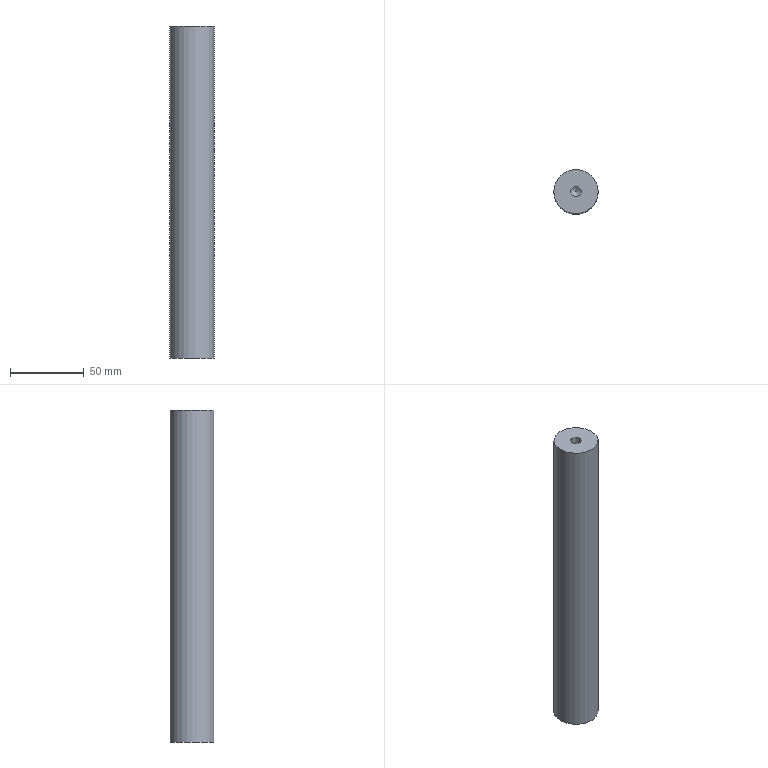Part | NX | features solid 2 | 1 solid | 7 faces | box 30 x 30 x 225 mm | volume 156299 mm3 | cylinder 3 | plane 2 | cone 2 | commonest cylinder face diameters 6.985 x1 8.782 x1 30 x1
STEP:
#1=CARTESIAN_POINT('',(243.507,265.,-170.));
#2=VERTEX_POINT('',#1);
#3=CARTESIAN_POINT('',(247.,265.,-170.));
#4=DIRECTION('',(0.,0.,-1.));
#5=DIRECTION('',(-1.,0.,0.));
#6=AXIS2_PLACEMENT_3D('',#3,#4,#5);
#7=CIRCLE('',#6,3.493);
#8=EDGE_CURVE('',#2,#2,#7,.T.);
#9=ORIENTED_EDGE('',*,*,#8,.T.);
#10=EDGE_LOOP('',(#9));
#11=FACE_BOUND('',#10,.T.);
#12=CARTESIAN_POINT('',(232.,265.,-170.));
#13=VERTEX_POINT('',#12);
#14=CARTESIAN_POINT('',(247.,265.,-170.));
#15=DIRECTION('',(0.,0.,-1.));
#16=DIRECTION('',(-1.,0.,0.));
#17=AXIS2_PLACEMENT_3D('',#14,#15,#16);
#18=CIRCLE('',#17,15.);
#19=EDGE_CURVE('',#13,#13,#18,.T.);
#20=ORIENTED_EDGE('',*,*,#19,.F.);
#21=EDGE_LOOP('',(#20));
#22=FACE_BOUND('',#21,.T.);
#23=CARTESIAN_POINT('',(247.,285.,-170.));
#24=DIRECTION('',(0.,0.,-1.));
#25=DIRECTION('',(-1.,0.,0.));
#26=AXIS2_PLACEMENT_3D('',#23,#24,#25);
#27=PLANE('',#26);
#28=ADVANCED_FACE('',(#11,#22),#27,.F.);
#29=CARTESIAN_POINT('',(232.,265.,-395.));
#30=VERTEX_POINT('',#29);
#31=CARTESIAN_POINT('',(247.,265.,-395.));
#32=DIRECTION('',(0.,0.,-1.));
#33=DIRECTION('',(-1.,0.,0.));
#34=AXIS2_PLACEMENT_3D('',#31,#32,#33);
#35=CIRCLE('',#34,15.);
#36=EDGE_CURVE('',#30,#30,#35,.T.);
#37=ORIENTED_EDGE('',*,*,#36,.F.);
#38=EDGE_LOOP('',(#37));
#39=FACE_BOUND('',#38,.T.);
#40=ORIENTED_EDGE('',*,*,#19,.T.);
#41=EDGE_LOOP('',(#40));
#42=FACE_BOUND('',#41,.T.);
#43=CARTESIAN_POINT('',(247.,265.,-250.));
#44=DIRECTION('',(0.,0.,-1.));
#45=DIRECTION('',(-1.,0.,0.));
#46=AXIS2_PLACEMENT_3D('',#43,#44,#45);
#47=CYLINDRICAL_SURFACE('',#46,15.);
#48=ADVANCED_FACE('',(#39,#42),#47,.T.);
#49=CARTESIAN_POINT('',(251.391,265.,-395.));
#50=VERTEX_POINT('',#49);
#51=CARTESIAN_POINT('',(247.,265.,-395.));
#52=DIRECTION('',(0.,0.,1.));
#53=DIRECTION('',(1.,0.,0.));
#54=AXIS2_PLACEMENT_3D('',#51,#52,#53);
#55=CIRCLE('',#54,4.391);
#56=EDGE_CURVE('',#50,#50,#55,.T.);
#57=ORIENTED_EDGE('',*,*,#56,.T.);
#58=EDGE_LOOP('',(#57));
#59=FACE_BOUND('',#58,.T.);
#60=ORIENTED_EDGE('',*,*,#36,.T.);
#61=EDGE_LOOP('',(#60));
#62=FACE_BOUND('',#61,.T.);
#63=CARTESIAN_POINT('',(247.,265.,-395.));
#64=DIRECTION('',(0.,0.,-1.));
#65=DIRECTION('',(-1.,0.,0.));
#66=AXIS2_PLACEMENT_3D('',#63,#64,#65);
#67=PLANE('',#66);
#68=ADVANCED_FACE('',(#59,#62),#67,.T.);
#69=CARTESIAN_POINT('',(243.507,265.,-200.));
#70=VERTEX_POINT('',#69);
#71=CARTESIAN_POINT('',(247.,265.,-200.));
#72=DIRECTION('',(0.,0.,-1.));
#73=DIRECTION('',(-1.,0.,0.));
#74=AXIS2_PLACEMENT_3D('',#71,#72,#73);
#75=CIRCLE('',#74,3.493);
#76=EDGE_CURVE('',#70,#70,#75,.T.);
#77=ORIENTED_EDGE('',*,*,#76,.F.);
#78=EDGE_LOOP('',(#77));
#79=FACE_BOUND('',#78,.T.);
#80=CARTESIAN_POINT('',(247.,265.,-202.099));
#81=VERTEX_POINT('',#80);
#82=VERTEX_LOOP('',#81);
#83=FACE_BOUND('',#82,.T.);
#84=CARTESIAN_POINT('',(247.,265.,-200.));
#85=DIRECTION('',(0.,0.,1.));
#86=DIRECTION('',(1.,0.,0.));
#87=AXIS2_PLACEMENT_3D('',#84,#85,#86);
#88=CONICAL_SURFACE('',#87,3.493,1.03);
#89=ADVANCED_FACE('',(#79,#83),#88,.F.);
#90=ORIENTED_EDGE('',*,*,#76,.T.);
#91=EDGE_LOOP('',(#90));
#92=FACE_BOUND('',#91,.T.);
#93=ORIENTED_EDGE('',*,*,#8,.F.);
#94=EDGE_LOOP('',(#93));
#95=FACE_BOUND('',#94,.T.);
#96=CARTESIAN_POINT('',(247.,265.,-170.));
#97=DIRECTION('',(0.,0.,-1.));
#98=DIRECTION('',(-1.,0.,0.));
#99=AXIS2_PLACEMENT_3D('',#96,#97,#98);
#100=CYLINDRICAL_SURFACE('',#99,3.493);
#101=ADVANCED_FACE('',(#92,#95),#100,.F.);
#102=CARTESIAN_POINT('',(251.391,265.,-370.));
#103=VERTEX_POINT('',#102);
#104=CARTESIAN_POINT('',(247.,265.,-370.));
#105=DIRECTION('',(0.,0.,1.));
#106=DIRECTION('',(1.,0.,0.));
#107=AXIS2_PLACEMENT_3D('',#104,#105,#106);
#108=CIRCLE('',#107,4.391);
#109=EDGE_CURVE('',#103,#103,#108,.T.);
#110=ORIENTED_EDGE('',*,*,#109,.F.);
#111=EDGE_LOOP('',(#110));
#112=FACE_BOUND('',#111,.T.);
#113=CARTESIAN_POINT('',(247.,265.,-367.362));
#114=VERTEX_POINT('',#113);
#115=VERTEX_LOOP('',#114);
#116=FACE_BOUND('',#115,.T.);
#117=CARTESIAN_POINT('',(247.,265.,-370.));
#118=DIRECTION('',(0.,0.,-1.));
#119=DIRECTION('',(-1.,0.,0.));
#120=AXIS2_PLACEMENT_3D('',#117,#118,#119);
#121=CONICAL_SURFACE('',#120,4.391,1.03);
#122=ADVANCED_FACE('',(#112,#116),#121,.F.);
#123=ORIENTED_EDGE('',*,*,#109,.T.);
#124=EDGE_LOOP('',(#123));
#125=FACE_BOUND('',#124,.T.);
#126=ORIENTED_EDGE('',*,*,#56,.F.);
#127=EDGE_LOOP('',(#126));
#128=FACE_BOUND('',#127,.T.);
#129=CARTESIAN_POINT('',(247.,265.,-395.));
#130=DIRECTION('',(0.,0.,1.));
#131=DIRECTION('',(1.,0.,0.));
#132=AXIS2_PLACEMENT_3D('',#129,#130,#131);
#133=CYLINDRICAL_SURFACE('',#132,4.391);
#134=ADVANCED_FACE('',(#125,#128),#133,.F.);
#135=CLOSED_SHELL('',(#28,#48,#68,#89,#101,#122,#134));
#136=MANIFOLD_SOLID_BREP('',#135);
#137=(LENGTH_UNIT()NAMED_UNIT(*)SI_UNIT(.MILLI.,.METRE.));
#138=UNCERTAINTY_MEASURE_WITH_UNIT(LENGTH_MEASURE(0.00001),#137,'','');
#139=(NAMED_UNIT(*)PLANE_ANGLE_UNIT()SI_UNIT($,.RADIAN.));
#140=(NAMED_UNIT(*)SI_UNIT($,.STERADIAN.)SOLID_ANGLE_UNIT());
#141=(GEOMETRIC_REPRESENTATION_CONTEXT(3)GLOBAL_UNCERTAINTY_ASSIGNED_CONTEXT((#138))GLOBAL_UNIT_ASSIGNED_CONTEXT((#137,#139,#140))REPRESENTATION_CONTEXT('',''));
#142=ADVANCED_BREP_SHAPE_REPRESENTATION('',(#136),#141);